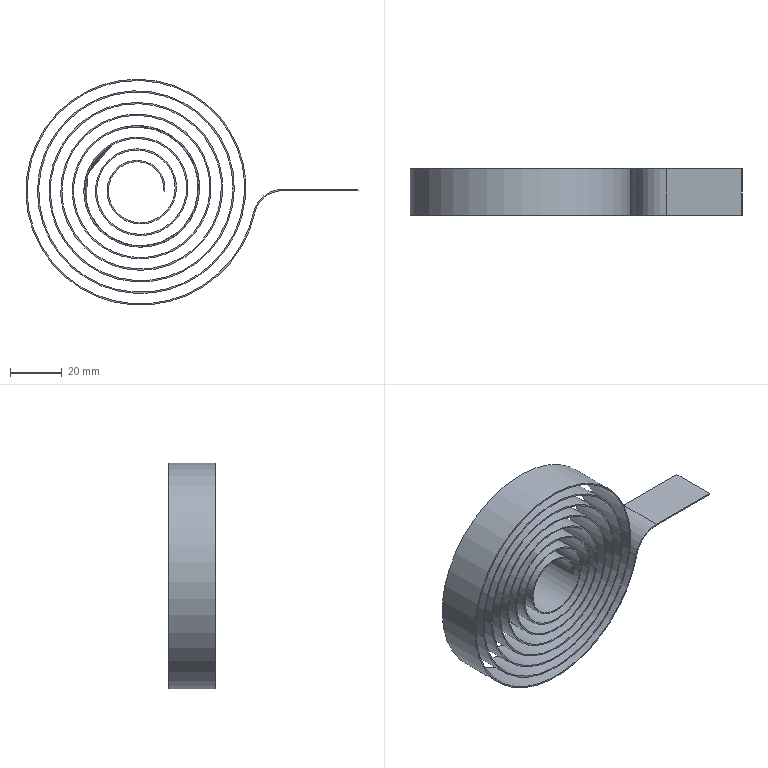Part | SolidWorks | features Helix 1, Sweep 1 | 1 solid | 14 faces | box 128.799 x 18 x 87.599 mm | volume 12839 mm3 | plane 10 | cylinder 2 | spline 2 | commonest cylinder face diameters 22.157 x1 23.157 x1